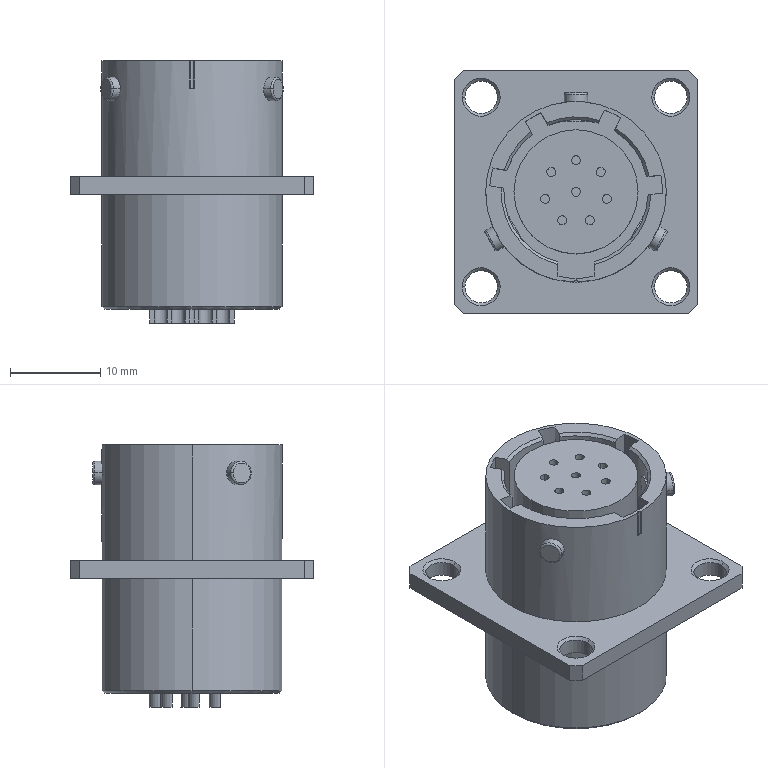Part | STEP file | Connector Y50X5-1208Z30K | 1 solid | 186 faces | box 27 x 27 x 29.03 mm | volume 7701 mm3 | cylinder 89 | plane 72 | cone 17 | torus 8 | commonest cylinder face diameters 2.6 x28 1 x16 2.5 x8 3.6 x8 1.5 x7 16 x5